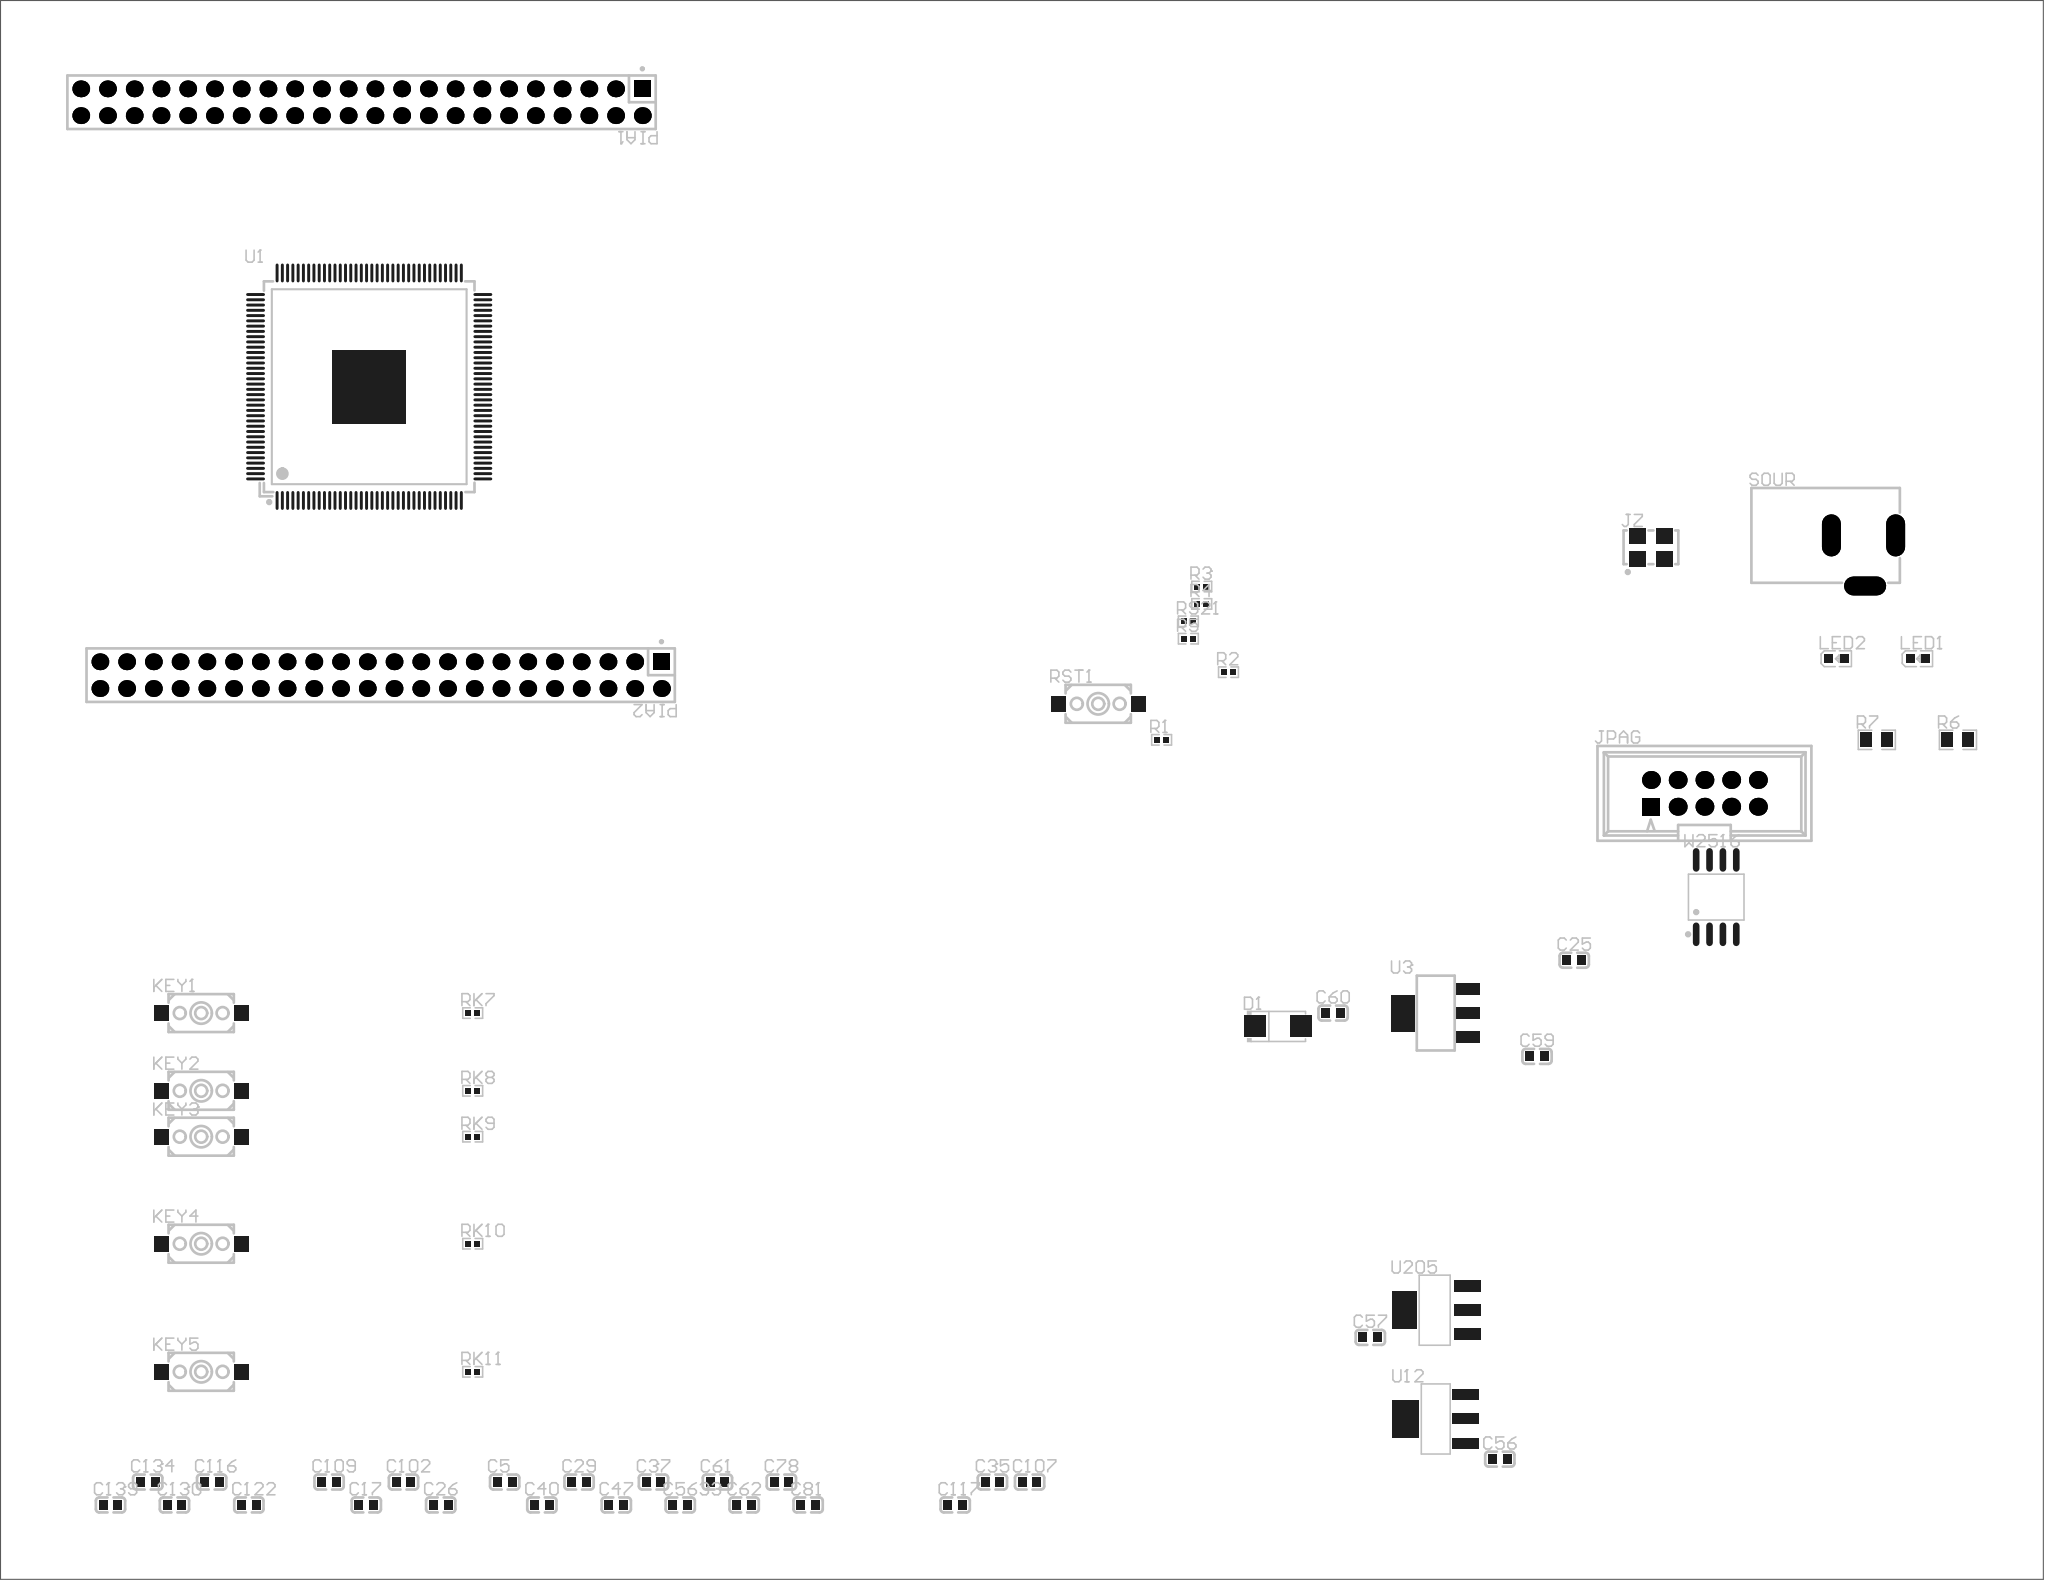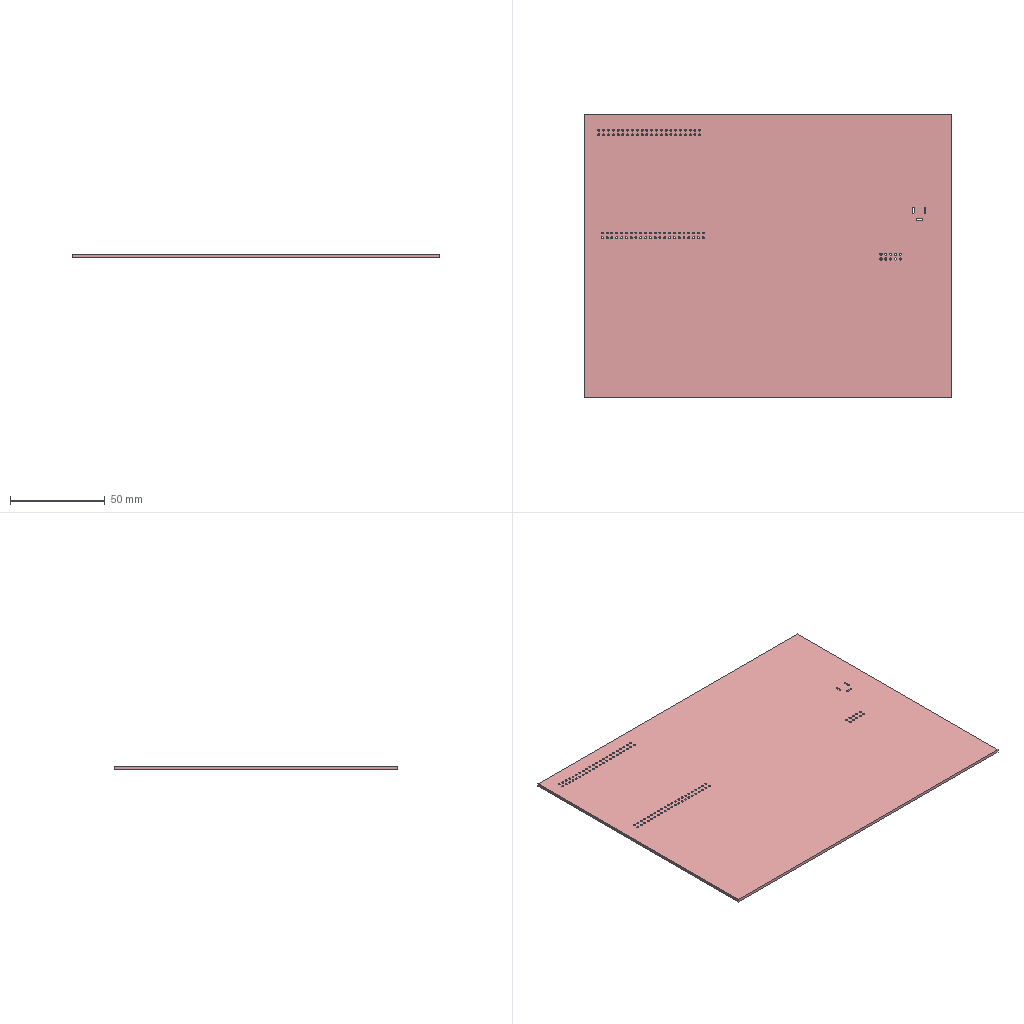Circuit board layout | Altium Designer | box 194 x 149.8 x 1.6 mm
Layer stack:
# Altium Designer layer stack of  (unit mm; dielectric type: 0 none, 1 core, 2 prepreg, 3 surface material)
index,name,kind,layer,copper_thickness_mm,dielectric_type,dielectric_thickness_mm,dielectric_material,dielectric_constant
0,Top Paste Mask Layer,other,,,,,,
1,Top Silkscreen Layer,other,,,,,,
2,Top Solder Mask Layer,dielectric,,,3,0.01,,3.3
3,Top Layer,copper,Top Layer,0.035,,,,
4,Dielectric1,dielectric,,,3,1.51,FR4,4.5
5,Bottom Layer,copper,Bottom Layer,0.035,,,,
6,Bottom Solder Mask Layer,dielectric,,,3,0.01,,3.3
7,Bottom Silkscreen Layer,other,,,,,,
8,Bottom Paste Mask Layer,other,,,,,,
# drill layer pairs: low layer,high layer
drill_pair,Top Layer,Bottom Layer
Part placement:
Designator,Comment,Layer,Footprint,Center-X(mm),Center-Y(mm),Rotation
C5,100nF,TopLayer,C0603,117.734,79.084,0
C17,100nF,TopLayer,C0603,104.592,76.91,0
C25,100nF,TopLayer,C0603,219.326,128.604,0
C26,100nF,TopLayer,C0603,111.66,76.91,0
C29,100nF,TopLayer,C0603,124.802,79.084,0
C35,100nF,TopLayer,C0603,164.062,79.084,0
C37,100nF,TopLayer,C0603,131.87,79.084,0
C40,100nF,TopLayer,C0603,121.268,76.91,0
C47,100nF,TopLayer,C0603,128.336,76.91,0
C56,10uF,TopLayer,C0603,212.258,81.258,0
C57,10uF,TopLayer,C0603,199.956,92.809,0
C59,10uF,TopLayer,C0603,215.792,119.478,0
C60,10uF,TopLayer,C0603,196.422,123.59,0
C61,100nF,TopLayer,C0603,137.944,79.084,0
C62,100nF,TopLayer,C0603,140.484,76.91,0
C78,100nF,TopLayer,C0603,144.018,79.084,0
C81,100nF,TopLayer,C0603,146.558,76.91,0
C102,100nF,TopLayer,C0603,108.126,79.084,0
C107,100nF,TopLayer,C0603,167.596,79.084,0
C109,100nF,TopLayer,C0603,101.058,79.084,0
C116,100nF,TopLayer,C0603,89.904,79.084,0
C117,100nF,TopLayer,C0603,160.528,76.91,0
C122,100nF,TopLayer,C0603,93.438,76.91,0
C130,100nF,TopLayer,C0603,86.37,76.91,0
C134,100nF,TopLayer,C0603,83.83,79.084,0
C139,100nF,TopLayer,C0603,80.296,76.91,0
C5633,100nF,TopLayer,C0603,134.41,76.91,0
D1,SMAJ5.0A-C83329,TopLayer,SMA_L4.3-W2.6-LS5.2-RD,191.205,122.32,0
JPAG,MTB110-10S,TopLayer,IDC-TH_MTB110-10S,231.693,144.441,0
JZ,50MHz,TopLayer,OSC-SMD_4P-L5.0-W3.2-BL_7CZ-XXXXX,226.613,167.793,0
KEY1,K2-3.6×6.1_SMD,TopLayer,KEY-SMD_2P-L6.2-W3.6-LS8.0,88.91,123.59,0
KEY2,K2-3.6×6.1_SMD,TopLayer,KEY-SMD_2P-L6.2-W3.6-LS8.0,88.91,116.214,0
KEY3,K2-3.6×6.1_SMD,TopLayer,KEY-SMD_2P-L6.2-W3.6-LS8.0,88.91,111.86,0
KEY4,K2-3.6×6.1_SMD,TopLayer,KEY-SMD_2P-L6.2-W3.6-LS8.0,88.91,101.7,0
KEY5,K2-3.6×6.1_SMD,TopLayer,KEY-SMD_2P-L6.2-W3.6-LS8.0,88.91,89.546,0
LED1,FC-1608YXK-585F08,TopLayer,LED0603-RD,251.969,157.213,0
LED2,FC-1608YXK-585F08,TopLayer,LED0603-RD,244.264,157.213,0
PIA1,X6521WV-2×22H-C30D60,TopLayer,HDR-TH_44P-2.54-V-M-R2-C22-S2.54,104.14,210.03,180
PIA2,X6521WV-2×22H-C30D60,TopLayer,HDR-TH_44P-2.54-V-M-R2-C22-S2.54,105.957,155.659,180
R1,10kΩ,TopLayer,R0402,180.133,149.521,0
R2,10kΩ,TopLayer,R0402,186.485,155.943,0
R3,10kΩ,TopLayer,R0402,183.944,164.068,0
R4,10kΩ,TopLayer,R0402,183.944,162.418,0
R5,10kΩ,TopLayer,R0402,182.674,159.119,0
R6,500Ω,TopLayer,R0805,255.772,149.521,0
R7,500Ω,TopLayer,R0805,248.067,149.521,0
R921,10kΩ,TopLayer,R0402,182.674,160.769,0
RK7,10kΩ,TopLayer,R0402,114.697,123.59,0
RK8,10kΩ,TopLayer,R0402,114.697,116.214,0
RK9,10kΩ,TopLayer,R0402,114.697,111.859,0
RK10,10kΩ,TopLayer,R0402,114.697,101.7,0
RK11,10kΩ,TopLayer,R0402,114.697,89.546,0
RST1,K2-3.6×6.1_SMD,TopLayer,KEY-SMD_2P-L6.2-W3.6-LS8.0,174.113,152.941,0
SOUR,DC-005-2.0_C22459640,TopLayer,DC-IN-TH_DC-005-2.0_C22459640,246.804,166.523,0
U1,EP4CE6E22C8N,TopLayer,PQFP-144_L20.0-W20.0-P0.50-LS22.0-BL-EP,104.868,183.033,0
U3,TLV1117LV33DCYR,TopLayer,SOT-223_L6.7-W3.5-P2.30-BR,206.172,123.59,0
U12,TLV1117LV12DCYR,TopLayer,SOT-223-4_L6.5-W3.5-P2.30-LS7.0-BR,206.172,85.068,0
U205,TLV1117LV25DCYR,TopLayer,SOT-223-3_L6.5-W3.4-P2.30-LS7.0-BR,206.172,95.392,0
W2516,W25Q16JVSSIQ,TopLayer,SOIC-8_L5.3-W5.3-P1.27-LS8.0-BL,232.812,134.596,0
Pad and via stacks:
# Altium Designer via and pad stacks of  (unit mm). Each distinct definition once, with the count of objects using it.
# via: kind,start_layer,end_layer,hole_mm,diameter_mm,mode(0 simple;1 top-mid-bottom;2 full stack),diameter_per_layer,count,example_net
# pad: kind,layer,hole_mm,hole_type(0 round;1 square;2 slot),plating,top_size,top_shape(1 round;2 rect;3 octagon;9 rounded rect),mid_size,bottom_size,mode,footprint,size_per_layer,count,example
pad,Top Layer,0,0,plated,0.8x0.9,2,0.8x0.9,0.8x0.9,0,C0603,,54,C5.2
pad,Top Layer,0,0,plated,2x2,2,2x2,2x2,0,SMA_L4.3-W2.6-LS5.2-RD,,2,D1.2
pad,Top Layer,0,0,plated,1.6x1.5,2,1.6x1.5,1.6x1.5,0,OSC-SMD_4P-L5.0-W3.2-BL_7CZ-XXXXX,,4,JZ.3
pad,Top Layer,0,0,plated,1.5x1.4,2,1.5x1.4,1.5x1.4,0,KEY-SMD_2P-L6.2-W3.6-LS8.0,,12,KEY1.1
pad,Top Layer,0,0,plated,0.8x0.8,2,0.8x0.8,0.8x0.8,0,LED0603-RD,,4,LED1.2
pad,Top Layer,0,0,plated,0.5657x0.54,2,0.5657x0.54,0.5657x0.54,0,R0402,,22,R1.2
pad,Top Layer,0,0,plated,1.133x1.377,2,1.133x1.377,1.133x1.377,0,R0805,,4,R6.2
pad,Top Layer,0,0,plated,0.28x1.8,1,0.28x1.8,0.28x1.8,0,PQFP-144_L20.0-W20.0-P0.50-LS22.0-BL-EP,,144,U1.1
pad,Top Layer,0,0,plated,7x7,2,7x7,7x7,0,PQFP-144_L20.0-W20.0-P0.50-LS22.0-BL-EP,,1,U1.145
pad,Top Layer,0,0,plated,2.2x3.5,2,2.2x3.5,2.2x3.5,0,SOT-223_L6.7-W3.5-P2.30-BR,,1,U3.4
pad,Top Layer,0,0,plated,1.1x2.2,2,1.1x2.2,1.1x2.2,0,SOT-223_L6.7-W3.5-P2.30-BR,,3,U3.3
pad,Top Layer,0,0,plated,2.47x0.98,2,2.47x0.98,2.47x0.98,0,SOT-223-4_L6.5-W3.5-P2.30-LS7.0-BR,,3,U12.1
pad,Top Layer,0,0,plated,2.47x3.6,2,2.47x3.6,2.47x3.6,0,SOT-223-4_L6.5-W3.5-P2.30-LS7.0-BR,,1,U12.4
pad,Top Layer,0,0,plated,2.5x1.1,2,2.5x1.1,2.5x1.1,0,SOT-223-3_L6.5-W3.4-P2.30-LS7.0-BR,,3,U205.1
pad,Top Layer,0,0,plated,2.34x3.6,2,2.34x3.6,2.34x3.6,0,SOT-223-3_L6.5-W3.4-P2.30-LS7.0-BR,,1,U205.4
pad,Top Layer,0,0,plated,0.63x2.25,1,0.63x2.25,0.63x2.25,0,SOIC-8_L5.3-W5.3-P1.27-LS8.0-BL,,8,W2516.1
pad,Multi-Layer,1.2,0,plated,1.7x1.7,2,1.7x1.7,1.7x1.7,0,IDC-TH_MTB110-10S,,1,JPAG.1
pad,Multi-Layer,1.2,0,plated,1.7x1.7,1,1.7x1.7,1.7x1.7,0,IDC-TH_MTB110-10S,,9,JPAG.2
pad,Multi-Layer,1.05,0,plated,1.6x1.6,2,1.6x1.6,1.6x1.6,0,HDR-TH_44P-2.54-V-M-R2-C22-S2.54,,2,PIA1.1
pad,Multi-Layer,1.05,0,plated,1.6x1.6,1,1.6x1.6,1.6x1.6,0,HDR-TH_44P-2.54-V-M-R2-C22-S2.54,,86,PIA1.2
pad,Multi-Layer,1,2,plated,4x1.8,1,4x1.8,4x1.8,0,DC-IN-TH_DC-005-2.0_C22459640,,3,SOUR.3